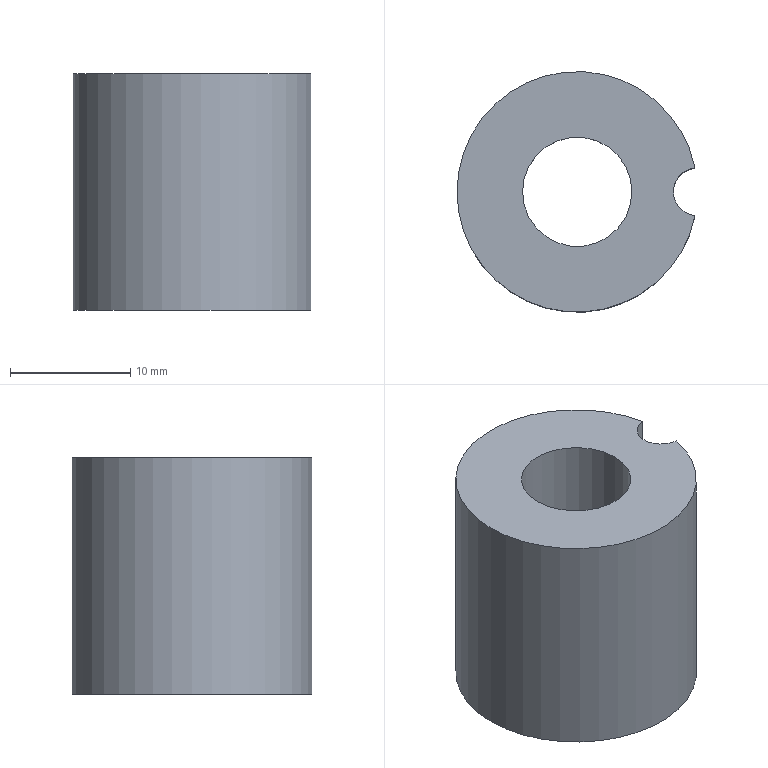Part | NX | features solid 2 | 1 solid | 7 faces | box 19.8 x 20 x 19.708 mm | volume 4075 mm3 | cylinder 4 | plane 3 | commonest cylinder face diameters 4 x1 9.1 x1 12.6 x1 20 x1
STEP:
#1=CARTESIAN_POINT('',(-120.211,-384.704,86.708));
#2=VERTEX_POINT('',#1);
#3=CARTESIAN_POINT('',(-120.211,-384.704,67.));
#4=VERTEX_POINT('',#3);
#5=CARTESIAN_POINT('',(-120.211,-384.704,77.));
#6=DIRECTION('',(0.,0.,1.));
#7=VECTOR('',#6,1000.);
#8=LINE('',#5,#7);
#9=EDGE_CURVE('',#2,#4,#8,.F.);
#10=ORIENTED_EDGE('',*,*,#9,.F.);
#11=CARTESIAN_POINT('',(-120.211,-380.724,86.708));
#12=VERTEX_POINT('',#11);
#13=CARTESIAN_POINT('',(-130.011,-382.714,86.708));
#14=DIRECTION('',(0.,0.,1.));
#15=DIRECTION('',(1.,0.,0.));
#16=AXIS2_PLACEMENT_3D('',#13,#14,#15);
#17=CIRCLE('',#16,10.);
#18=EDGE_CURVE('',#2,#12,#17,.F.);
#19=ORIENTED_EDGE('',*,*,#18,.T.);
#20=CARTESIAN_POINT('',(-120.211,-380.724,67.));
#21=VERTEX_POINT('',#20);
#22=CARTESIAN_POINT('',(-120.211,-380.724,77.));
#23=DIRECTION('',(0.,0.,1.));
#24=VECTOR('',#23,1000.);
#25=LINE('',#22,#24);
#26=EDGE_CURVE('',#21,#12,#25,.T.);
#27=ORIENTED_EDGE('',*,*,#26,.F.);
#28=CARTESIAN_POINT('',(-130.011,-382.714,67.));
#29=DIRECTION('',(0.,0.,1.));
#30=DIRECTION('',(1.,0.,0.));
#31=AXIS2_PLACEMENT_3D('',#28,#29,#30);
#32=CIRCLE('',#31,10.);
#33=EDGE_CURVE('',#21,#4,#32,.T.);
#34=ORIENTED_EDGE('',*,*,#33,.T.);
#35=EDGE_LOOP('',(#10,#19,#27,#34));
#36=FACE_BOUND('',#35,.T.);
#37=CARTESIAN_POINT('',(-130.011,-382.714,67.));
#38=DIRECTION('',(0.,0.,1.));
#39=DIRECTION('',(1.,0.,0.));
#40=AXIS2_PLACEMENT_3D('',#37,#38,#39);
#41=CYLINDRICAL_SURFACE('',#40,10.);
#42=ADVANCED_FACE('',(#36),#41,.T.);
#43=CARTESIAN_POINT('',(-120.011,-382.714,86.708));
#44=DIRECTION('',(0.,0.,1.));
#45=DIRECTION('',(1.,0.,0.));
#46=AXIS2_PLACEMENT_3D('',#43,#44,#45);
#47=CIRCLE('',#46,2.);
#48=EDGE_CURVE('',#2,#12,#47,.F.);
#49=ORIENTED_EDGE('',*,*,#48,.F.);
#50=ORIENTED_EDGE('',*,*,#9,.T.);
#51=CARTESIAN_POINT('',(-120.011,-382.714,67.));
#52=DIRECTION('',(0.,0.,1.));
#53=DIRECTION('',(1.,0.,0.));
#54=AXIS2_PLACEMENT_3D('',#51,#52,#53);
#55=CIRCLE('',#54,2.);
#56=EDGE_CURVE('',#21,#4,#55,.T.);
#57=ORIENTED_EDGE('',*,*,#56,.F.);
#58=ORIENTED_EDGE('',*,*,#26,.T.);
#59=EDGE_LOOP('',(#49,#50,#57,#58));
#60=FACE_BOUND('',#59,.T.);
#61=CARTESIAN_POINT('',(-120.011,-382.714,67.));
#62=DIRECTION('',(0.,0.,1.));
#63=DIRECTION('',(1.,0.,0.));
#64=AXIS2_PLACEMENT_3D('',#61,#62,#63);
#65=CYLINDRICAL_SURFACE('',#64,2.);
#66=ADVANCED_FACE('',(#60),#65,.F.);
#67=CARTESIAN_POINT('',(-125.461,-382.714,79.));
#68=VERTEX_POINT('',#67);
#69=CARTESIAN_POINT('',(-130.011,-382.714,79.));
#70=DIRECTION('',(0.,0.,1.));
#71=DIRECTION('',(1.,0.,0.));
#72=AXIS2_PLACEMENT_3D('',#69,#70,#71);
#73=CIRCLE('',#72,4.55);
#74=EDGE_CURVE('',#68,#68,#73,.T.);
#75=ORIENTED_EDGE('',*,*,#74,.F.);
#76=EDGE_LOOP('',(#75));
#77=FACE_BOUND('',#76,.T.);
#78=CARTESIAN_POINT('',(-125.461,-382.714,86.708));
#79=VERTEX_POINT('',#78);
#80=CARTESIAN_POINT('',(-130.011,-382.714,86.708));
#81=DIRECTION('',(0.,0.,1.));
#82=DIRECTION('',(1.,0.,0.));
#83=AXIS2_PLACEMENT_3D('',#80,#81,#82);
#84=CIRCLE('',#83,4.55);
#85=EDGE_CURVE('',#79,#79,#84,.F.);
#86=ORIENTED_EDGE('',*,*,#85,.F.);
#87=EDGE_LOOP('',(#86));
#88=FACE_BOUND('',#87,.T.);
#89=CARTESIAN_POINT('',(-130.011,-382.714,67.));
#90=DIRECTION('',(0.,0.,1.));
#91=DIRECTION('',(1.,0.,0.));
#92=AXIS2_PLACEMENT_3D('',#89,#90,#91);
#93=CYLINDRICAL_SURFACE('',#92,4.55);
#94=ADVANCED_FACE('',(#77,#88),#93,.F.);
#95=CARTESIAN_POINT('',(-123.711,-382.714,67.));
#96=VERTEX_POINT('',#95);
#97=CARTESIAN_POINT('',(-130.011,-382.714,67.));
#98=DIRECTION('',(0.,0.,1.));
#99=DIRECTION('',(1.,0.,0.));
#100=AXIS2_PLACEMENT_3D('',#97,#98,#99);
#101=CIRCLE('',#100,6.3);
#102=EDGE_CURVE('',#96,#96,#101,.T.);
#103=ORIENTED_EDGE('',*,*,#102,.T.);
#104=EDGE_LOOP('',(#103));
#105=FACE_BOUND('',#104,.T.);
#106=ORIENTED_EDGE('',*,*,#33,.F.);
#107=ORIENTED_EDGE('',*,*,#56,.T.);
#108=EDGE_LOOP('',(#106,#107));
#109=FACE_BOUND('',#108,.T.);
#110=CARTESIAN_POINT('',(-130.011,-382.714,67.));
#111=DIRECTION('',(0.,0.,1.));
#112=DIRECTION('',(1.,0.,0.));
#113=AXIS2_PLACEMENT_3D('',#110,#111,#112);
#114=PLANE('',#113);
#115=ADVANCED_FACE('',(#105,#109),#114,.F.);
#116=ORIENTED_EDGE('',*,*,#102,.F.);
#117=EDGE_LOOP('',(#116));
#118=FACE_BOUND('',#117,.T.);
#119=CARTESIAN_POINT('',(-123.711,-382.714,79.));
#120=VERTEX_POINT('',#119);
#121=CARTESIAN_POINT('',(-130.011,-382.714,79.));
#122=DIRECTION('',(0.,0.,1.));
#123=DIRECTION('',(1.,0.,0.));
#124=AXIS2_PLACEMENT_3D('',#121,#122,#123);
#125=CIRCLE('',#124,6.3);
#126=EDGE_CURVE('',#120,#120,#125,.T.);
#127=ORIENTED_EDGE('',*,*,#126,.T.);
#128=EDGE_LOOP('',(#127));
#129=FACE_BOUND('',#128,.T.);
#130=CARTESIAN_POINT('',(-130.011,-382.714,67.));
#131=DIRECTION('',(0.,0.,1.));
#132=DIRECTION('',(1.,0.,0.));
#133=AXIS2_PLACEMENT_3D('',#130,#131,#132);
#134=CYLINDRICAL_SURFACE('',#133,6.3);
#135=ADVANCED_FACE('',(#118,#129),#134,.F.);
#136=ORIENTED_EDGE('',*,*,#74,.T.);
#137=EDGE_LOOP('',(#136));
#138=FACE_BOUND('',#137,.T.);
#139=ORIENTED_EDGE('',*,*,#126,.F.);
#140=EDGE_LOOP('',(#139));
#141=FACE_BOUND('',#140,.T.);
#142=CARTESIAN_POINT('',(-130.011,-382.714,79.));
#143=DIRECTION('',(0.,0.,1.));
#144=DIRECTION('',(1.,0.,0.));
#145=AXIS2_PLACEMENT_3D('',#142,#143,#144);
#146=PLANE('',#145);
#147=ADVANCED_FACE('',(#138,#141),#146,.F.);
#148=ORIENTED_EDGE('',*,*,#18,.F.);
#149=ORIENTED_EDGE('',*,*,#48,.T.);
#150=EDGE_LOOP('',(#148,#149));
#151=FACE_BOUND('',#150,.T.);
#152=ORIENTED_EDGE('',*,*,#85,.T.);
#153=EDGE_LOOP('',(#152));
#154=FACE_BOUND('',#153,.T.);
#155=CARTESIAN_POINT('',(426.488,227.578,86.708));
#156=DIRECTION('',(0.,0.,1.));
#157=DIRECTION('',(0.,-1.,0.));
#158=AXIS2_PLACEMENT_3D('',#155,#156,#157);
#159=PLANE('',#158);
#160=ADVANCED_FACE('',(#151,#154),#159,.T.);
#161=CLOSED_SHELL('',(#42,#66,#94,#115,#135,#147,#160));
#162=MANIFOLD_SOLID_BREP('',#161);
#163=(LENGTH_UNIT()NAMED_UNIT(*)SI_UNIT(.MILLI.,.METRE.));
#164=UNCERTAINTY_MEASURE_WITH_UNIT(LENGTH_MEASURE(0.00001),#163,'','');
#165=(NAMED_UNIT(*)PLANE_ANGLE_UNIT()SI_UNIT($,.RADIAN.));
#166=(NAMED_UNIT(*)SI_UNIT($,.STERADIAN.)SOLID_ANGLE_UNIT());
#167=(GEOMETRIC_REPRESENTATION_CONTEXT(3)GLOBAL_UNCERTAINTY_ASSIGNED_CONTEXT((#164))GLOBAL_UNIT_ASSIGNED_CONTEXT((#163,#165,#166))REPRESENTATION_CONTEXT('',''));
#168=ADVANCED_BREP_SHAPE_REPRESENTATION('',(#162),#167);